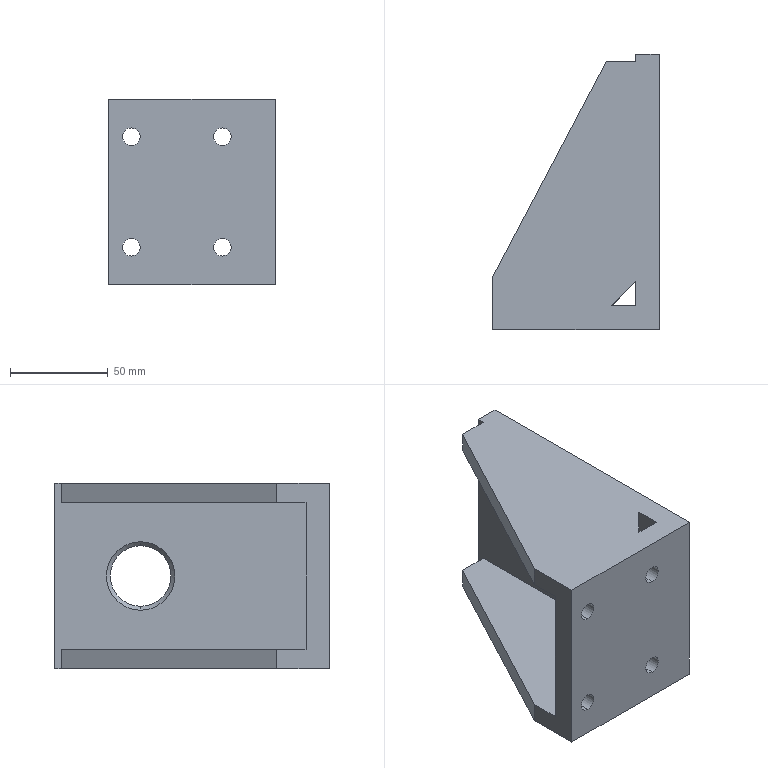Part | STEP file | YCD14007A-08.02.03-Lift Cylinder Seat-A3 | 1 solid | 30 faces | box 85 x 140.5 x 95 mm | volume 348010 mm3 | plane 16 | cylinder 10 | cone 4 | commonest cylinder face diameters 9 x8 31 x2